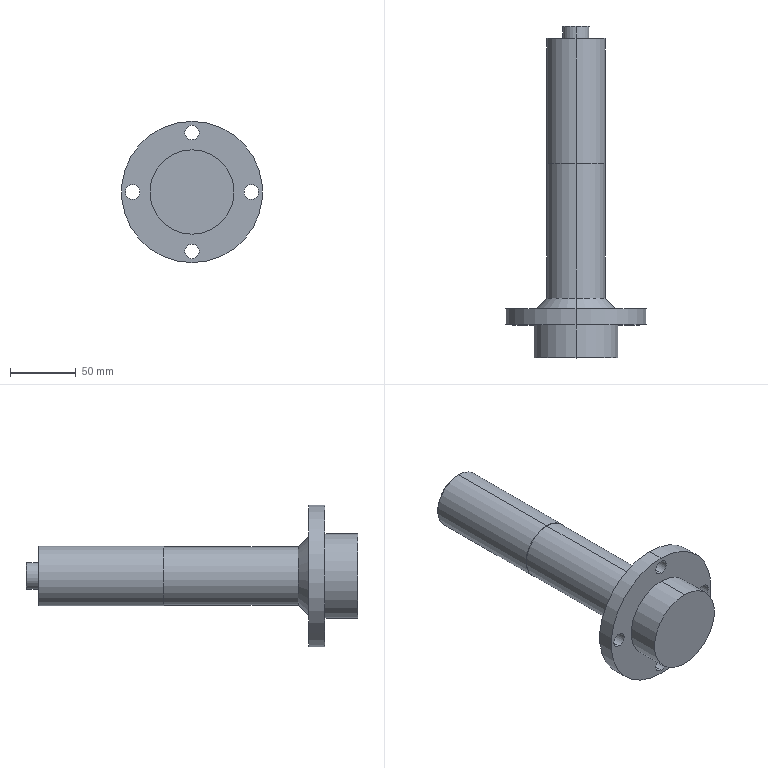Part | SolidWorks | features BaseBody 1 | 1 solid | 46 faces | box 107 x 251.6 x 107 mm | volume 513501 mm3 | cylinder 26 | cone 14 | plane 6 | commonest cylinder face diameters 5 x8 11 x8 20 x2 44.3 x2 45 x2 64 x2
STEP:
#1=CARTESIAN_POINT('',(0.,147.3,-22.15));
#2=VERTEX_POINT('',#1);
#3=CARTESIAN_POINT('',(0.,147.3,22.15));
#4=VERTEX_POINT('',#3);
#5=CARTESIAN_POINT('',(0.,147.3,0.));
#6=DIRECTION('',(0.,-1.,0.));
#7=DIRECTION('',(0.,0.,-1.));
#8=AXIS2_PLACEMENT_3D('',#5,#6,#7);
#9=CIRCLE('',#8,22.15);
#10=EDGE_CURVE('',#2,#4,#9,.T.);
#11=ORIENTED_EDGE('',*,*,#10,.T.);
#12=CARTESIAN_POINT('',(0.,45.3,22.15));
#13=VERTEX_POINT('',#12);
#14=CARTESIAN_POINT('',(0.,147.3,22.15));
#15=DIRECTION('',(0.,-1.,0.));
#16=VECTOR('',#15,1000.);
#17=LINE('',#14,#16);
#18=EDGE_CURVE('',#4,#13,#17,.T.);
#19=ORIENTED_EDGE('',*,*,#18,.T.);
#20=CARTESIAN_POINT('',(0.,45.3,-22.15));
#21=VERTEX_POINT('',#20);
#22=CARTESIAN_POINT('',(0.,45.3,0.));
#23=DIRECTION('',(0.,1.,0.));
#24=DIRECTION('',(0.,0.,-1.));
#25=AXIS2_PLACEMENT_3D('',#22,#23,#24);
#26=CIRCLE('',#25,22.15);
#27=EDGE_CURVE('',#13,#21,#26,.T.);
#28=ORIENTED_EDGE('',*,*,#27,.T.);
#29=CARTESIAN_POINT('',(0.,147.3,-22.15));
#30=DIRECTION('',(0.,-1.,0.));
#31=VECTOR('',#30,1000.);
#32=LINE('',#29,#31);
#33=EDGE_CURVE('',#2,#21,#32,.T.);
#34=ORIENTED_EDGE('',*,*,#33,.F.);
#35=EDGE_LOOP('',(#11,#19,#28,#34));
#36=FACE_OUTER_BOUND('',#35,.T.);
#37=CARTESIAN_POINT('',(0.,147.3,0.));
#38=DIRECTION('',(0.,-1.,0.));
#39=DIRECTION('',(0.,0.,-1.));
#40=AXIS2_PLACEMENT_3D('',#37,#38,#39);
#41=CYLINDRICAL_SURFACE('',#40,22.15);
#42=ADVANCED_FACE('',(#36),#41,.T.);
#43=ORIENTED_EDGE('',*,*,#27,.F.);
#44=CARTESIAN_POINT('',(0.,37.3,30.15));
#45=VERTEX_POINT('',#44);
#46=CARTESIAN_POINT('',(0.,37.3,30.15));
#47=DIRECTION('',(0.,-0.7071,0.7071));
#48=VECTOR('',#47,1000.);
#49=LINE('',#46,#48);
#50=EDGE_CURVE('',#13,#45,#49,.T.);
#51=ORIENTED_EDGE('',*,*,#50,.T.);
#52=CARTESIAN_POINT('',(0.,37.3,-30.15));
#53=VERTEX_POINT('',#52);
#54=CARTESIAN_POINT('',(0.,37.3,0.));
#55=DIRECTION('',(0.,1.,0.));
#56=DIRECTION('',(0.,0.,-1.));
#57=AXIS2_PLACEMENT_3D('',#54,#55,#56);
#58=CIRCLE('',#57,30.15);
#59=EDGE_CURVE('',#45,#53,#58,.T.);
#60=ORIENTED_EDGE('',*,*,#59,.T.);
#61=CARTESIAN_POINT('',(0.,37.3,-30.15));
#62=DIRECTION('',(0.,-0.7071,-0.7071));
#63=VECTOR('',#62,1000.);
#64=LINE('',#61,#63);
#65=EDGE_CURVE('',#21,#53,#64,.T.);
#66=ORIENTED_EDGE('',*,*,#65,.F.);
#67=EDGE_LOOP('',(#43,#51,#60,#66));
#68=FACE_OUTER_BOUND('',#67,.T.);
#69=CARTESIAN_POINT('',(0.,37.3,0.));
#70=DIRECTION('',(0.,-1.,0.));
#71=DIRECTION('',(0.,0.,-1.));
#72=AXIS2_PLACEMENT_3D('',#69,#70,#71);
#73=CONICAL_SURFACE('',#72,30.15,0.7854);
#74=ADVANCED_FACE('',(#68),#73,.T.);
#75=CARTESIAN_POINT('',(0.,241.8,-22.5));
#76=VERTEX_POINT('',#75);
#77=CARTESIAN_POINT('',(0.,241.8,22.5));
#78=VERTEX_POINT('',#77);
#79=CARTESIAN_POINT('',(0.,241.8,0.));
#80=DIRECTION('',(0.,-1.,0.));
#81=DIRECTION('',(0.,0.,-1.));
#82=AXIS2_PLACEMENT_3D('',#79,#80,#81);
#83=CIRCLE('',#82,22.5);
#84=EDGE_CURVE('',#76,#78,#83,.T.);
#85=ORIENTED_EDGE('',*,*,#84,.T.);
#86=CARTESIAN_POINT('',(0.,147.3,22.5));
#87=VERTEX_POINT('',#86);
#88=CARTESIAN_POINT('',(0.,242.3,22.5));
#89=DIRECTION('',(0.,-1.,0.));
#90=VECTOR('',#89,1000.);
#91=LINE('',#88,#90);
#92=EDGE_CURVE('',#78,#87,#91,.T.);
#93=ORIENTED_EDGE('',*,*,#92,.T.);
#94=CARTESIAN_POINT('',(0.,147.3,-22.5));
#95=VERTEX_POINT('',#94);
#96=CARTESIAN_POINT('',(0.,147.3,0.));
#97=DIRECTION('',(0.,1.,0.));
#98=DIRECTION('',(0.,0.,-1.));
#99=AXIS2_PLACEMENT_3D('',#96,#97,#98);
#100=CIRCLE('',#99,22.5);
#101=EDGE_CURVE('',#87,#95,#100,.T.);
#102=ORIENTED_EDGE('',*,*,#101,.T.);
#103=CARTESIAN_POINT('',(0.,242.3,-22.5));
#104=DIRECTION('',(0.,-1.,0.));
#105=VECTOR('',#104,1000.);
#106=LINE('',#103,#105);
#107=EDGE_CURVE('',#76,#95,#106,.T.);
#108=ORIENTED_EDGE('',*,*,#107,.F.);
#109=EDGE_LOOP('',(#85,#93,#102,#108));
#110=FACE_OUTER_BOUND('',#109,.T.);
#111=CARTESIAN_POINT('',(0.,242.3,0.));
#112=DIRECTION('',(0.,-1.,0.));
#113=DIRECTION('',(0.,0.,-1.));
#114=AXIS2_PLACEMENT_3D('',#111,#112,#113);
#115=CYLINDRICAL_SURFACE('',#114,22.5);
#116=ADVANCED_FACE('',(#110),#115,.T.);
#117=CARTESIAN_POINT('',(0.,37.3,53.5));
#118=VERTEX_POINT('',#117);
#119=CARTESIAN_POINT('',(0.,37.3,-53.5));
#120=VERTEX_POINT('',#119);
#121=CARTESIAN_POINT('',(0.,37.3,0.));
#122=DIRECTION('',(0.,1.,0.));
#123=DIRECTION('',(0.,0.,-1.));
#124=AXIS2_PLACEMENT_3D('',#121,#122,#123);
#125=CIRCLE('',#124,53.5);
#126=EDGE_CURVE('',#118,#120,#125,.T.);
#127=ORIENTED_EDGE('',*,*,#126,.F.);
#128=CARTESIAN_POINT('',(0.,25.,53.5));
#129=VERTEX_POINT('',#128);
#130=CARTESIAN_POINT('',(0.,37.3,53.5));
#131=DIRECTION('',(0.,-1.,0.));
#132=VECTOR('',#131,1000.);
#133=LINE('',#130,#132);
#134=EDGE_CURVE('',#118,#129,#133,.T.);
#135=ORIENTED_EDGE('',*,*,#134,.T.);
#136=CARTESIAN_POINT('',(0.,25.,-53.5));
#137=VERTEX_POINT('',#136);
#138=CARTESIAN_POINT('',(0.,25.,0.));
#139=DIRECTION('',(0.,1.,0.));
#140=DIRECTION('',(0.,0.,-1.));
#141=AXIS2_PLACEMENT_3D('',#138,#139,#140);
#142=CIRCLE('',#141,53.5);
#143=EDGE_CURVE('',#129,#137,#142,.T.);
#144=ORIENTED_EDGE('',*,*,#143,.T.);
#145=CARTESIAN_POINT('',(0.,37.3,-53.5));
#146=DIRECTION('',(0.,-1.,0.));
#147=VECTOR('',#146,1000.);
#148=LINE('',#145,#147);
#149=EDGE_CURVE('',#120,#137,#148,.T.);
#150=ORIENTED_EDGE('',*,*,#149,.F.);
#151=EDGE_LOOP('',(#127,#135,#144,#150));
#152=FACE_OUTER_BOUND('',#151,.T.);
#153=CARTESIAN_POINT('',(0.,37.3,0.));
#154=DIRECTION('',(0.,-1.,0.));
#155=DIRECTION('',(0.,0.,-1.));
#156=AXIS2_PLACEMENT_3D('',#153,#154,#155);
#157=CYLINDRICAL_SURFACE('',#156,53.5);
#158=ADVANCED_FACE('',(#152),#157,.T.);
#159=CARTESIAN_POINT('',(-45.,37.3,5.5));
#160=VERTEX_POINT('',#159);
#161=CARTESIAN_POINT('',(-45.,37.3,-5.5));
#162=VERTEX_POINT('',#161);
#163=CARTESIAN_POINT('',(-45.,37.3,0.));
#164=DIRECTION('',(0.,-1.,0.));
#165=DIRECTION('',(0.,0.,-1.));
#166=AXIS2_PLACEMENT_3D('',#163,#164,#165);
#167=CIRCLE('',#166,5.5);
#168=EDGE_CURVE('',#160,#162,#167,.T.);
#169=ORIENTED_EDGE('',*,*,#168,.F.);
#170=CARTESIAN_POINT('',(-45.,25.,5.5));
#171=VERTEX_POINT('',#170);
#172=CARTESIAN_POINT('',(-45.,37.3,5.5));
#173=DIRECTION('',(0.,-1.,0.));
#174=VECTOR('',#173,1000.);
#175=LINE('',#172,#174);
#176=EDGE_CURVE('',#160,#171,#175,.T.);
#177=ORIENTED_EDGE('',*,*,#176,.T.);
#178=CARTESIAN_POINT('',(-45.,25.,-5.5));
#179=VERTEX_POINT('',#178);
#180=CARTESIAN_POINT('',(-45.,25.,0.));
#181=DIRECTION('',(0.,1.,0.));
#182=DIRECTION('',(0.,0.,-1.));
#183=AXIS2_PLACEMENT_3D('',#180,#181,#182);
#184=CIRCLE('',#183,5.5);
#185=EDGE_CURVE('',#179,#171,#184,.T.);
#186=ORIENTED_EDGE('',*,*,#185,.F.);
#187=CARTESIAN_POINT('',(-45.,37.3,-5.5));
#188=DIRECTION('',(0.,-1.,0.));
#189=VECTOR('',#188,1000.);
#190=LINE('',#187,#189);
#191=EDGE_CURVE('',#162,#179,#190,.T.);
#192=ORIENTED_EDGE('',*,*,#191,.F.);
#193=EDGE_LOOP('',(#169,#177,#186,#192));
#194=FACE_OUTER_BOUND('',#193,.T.);
#195=CARTESIAN_POINT('',(-45.,37.3,0.));
#196=DIRECTION('',(0.,-1.,0.));
#197=DIRECTION('',(0.,0.,-1.));
#198=AXIS2_PLACEMENT_3D('',#195,#196,#197);
#199=CYLINDRICAL_SURFACE('',#198,5.5);
#200=ADVANCED_FACE('',(#194),#199,.F.);
#201=CARTESIAN_POINT('',(0.,37.3,-39.5));
#202=VERTEX_POINT('',#201);
#203=CARTESIAN_POINT('',(0.,37.3,-50.5));
#204=VERTEX_POINT('',#203);
#205=CARTESIAN_POINT('',(0.,37.3,-45.));
#206=DIRECTION('',(0.,-1.,0.));
#207=DIRECTION('',(0.,0.,-1.));
#208=AXIS2_PLACEMENT_3D('',#205,#206,#207);
#209=CIRCLE('',#208,5.5);
#210=EDGE_CURVE('',#202,#204,#209,.T.);
#211=ORIENTED_EDGE('',*,*,#210,.F.);
#212=CARTESIAN_POINT('',(0.,25.,-39.5));
#213=VERTEX_POINT('',#212);
#214=CARTESIAN_POINT('',(0.,37.3,-39.5));
#215=DIRECTION('',(0.,-1.,0.));
#216=VECTOR('',#215,1000.);
#217=LINE('',#214,#216);
#218=EDGE_CURVE('',#202,#213,#217,.T.);
#219=ORIENTED_EDGE('',*,*,#218,.T.);
#220=CARTESIAN_POINT('',(0.,25.,-50.5));
#221=VERTEX_POINT('',#220);
#222=CARTESIAN_POINT('',(0.,25.,-45.));
#223=DIRECTION('',(0.,1.,0.));
#224=DIRECTION('',(0.,0.,-1.));
#225=AXIS2_PLACEMENT_3D('',#222,#223,#224);
#226=CIRCLE('',#225,5.5);
#227=EDGE_CURVE('',#221,#213,#226,.T.);
#228=ORIENTED_EDGE('',*,*,#227,.F.);
#229=CARTESIAN_POINT('',(0.,37.3,-50.5));
#230=DIRECTION('',(0.,-1.,0.));
#231=VECTOR('',#230,1000.);
#232=LINE('',#229,#231);
#233=EDGE_CURVE('',#204,#221,#232,.T.);
#234=ORIENTED_EDGE('',*,*,#233,.F.);
#235=EDGE_LOOP('',(#211,#219,#228,#234));
#236=FACE_OUTER_BOUND('',#235,.T.);
#237=CARTESIAN_POINT('',(0.,37.3,-45.));
#238=DIRECTION('',(0.,-1.,0.));
#239=DIRECTION('',(0.,0.,-1.));
#240=AXIS2_PLACEMENT_3D('',#237,#238,#239);
#241=CYLINDRICAL_SURFACE('',#240,5.5);
#242=ADVANCED_FACE('',(#236),#241,.F.);
#243=CARTESIAN_POINT('',(45.,37.3,5.5));
#244=VERTEX_POINT('',#243);
#245=CARTESIAN_POINT('',(45.,37.3,-5.5));
#246=VERTEX_POINT('',#245);
#247=CARTESIAN_POINT('',(45.,37.3,0.));
#248=DIRECTION('',(0.,-1.,0.));
#249=DIRECTION('',(0.,0.,-1.));
#250=AXIS2_PLACEMENT_3D('',#247,#248,#249);
#251=CIRCLE('',#250,5.5);
#252=EDGE_CURVE('',#244,#246,#251,.T.);
#253=ORIENTED_EDGE('',*,*,#252,.F.);
#254=CARTESIAN_POINT('',(45.,25.,5.5));
#255=VERTEX_POINT('',#254);
#256=CARTESIAN_POINT('',(45.,37.3,5.5));
#257=DIRECTION('',(0.,-1.,0.));
#258=VECTOR('',#257,1000.);
#259=LINE('',#256,#258);
#260=EDGE_CURVE('',#244,#255,#259,.T.);
#261=ORIENTED_EDGE('',*,*,#260,.T.);
#262=CARTESIAN_POINT('',(45.,25.,-5.5));
#263=VERTEX_POINT('',#262);
#264=CARTESIAN_POINT('',(45.,25.,0.));
#265=DIRECTION('',(0.,1.,0.));
#266=DIRECTION('',(0.,0.,-1.));
#267=AXIS2_PLACEMENT_3D('',#264,#265,#266);
#268=CIRCLE('',#267,5.5);
#269=EDGE_CURVE('',#263,#255,#268,.T.);
#270=ORIENTED_EDGE('',*,*,#269,.F.);
#271=CARTESIAN_POINT('',(45.,37.3,-5.5));
#272=DIRECTION('',(0.,-1.,0.));
#273=VECTOR('',#272,1000.);
#274=LINE('',#271,#273);
#275=EDGE_CURVE('',#246,#263,#274,.T.);
#276=ORIENTED_EDGE('',*,*,#275,.F.);
#277=EDGE_LOOP('',(#253,#261,#270,#276));
#278=FACE_OUTER_BOUND('',#277,.T.);
#279=CARTESIAN_POINT('',(45.,37.3,0.));
#280=DIRECTION('',(0.,-1.,0.));
#281=DIRECTION('',(0.,0.,-1.));
#282=AXIS2_PLACEMENT_3D('',#279,#280,#281);
#283=CYLINDRICAL_SURFACE('',#282,5.5);
#284=ADVANCED_FACE('',(#278),#283,.F.);
#285=CARTESIAN_POINT('',(0.,37.3,50.5));
#286=VERTEX_POINT('',#285);
#287=CARTESIAN_POINT('',(0.,37.3,39.5));
#288=VERTEX_POINT('',#287);
#289=CARTESIAN_POINT('',(0.,37.3,45.));
#290=DIRECTION('',(0.,-1.,0.));
#291=DIRECTION('',(0.,0.,-1.));
#292=AXIS2_PLACEMENT_3D('',#289,#290,#291);
#293=CIRCLE('',#292,5.5);
#294=EDGE_CURVE('',#286,#288,#293,.T.);
#295=ORIENTED_EDGE('',*,*,#294,.F.);
#296=CARTESIAN_POINT('',(0.,25.,50.5));
#297=VERTEX_POINT('',#296);
#298=CARTESIAN_POINT('',(0.,37.3,50.5));
#299=DIRECTION('',(0.,-1.,0.));
#300=VECTOR('',#299,1000.);
#301=LINE('',#298,#300);
#302=EDGE_CURVE('',#286,#297,#301,.T.);
#303=ORIENTED_EDGE('',*,*,#302,.T.);
#304=CARTESIAN_POINT('',(0.,25.,39.5));
#305=VERTEX_POINT('',#304);
#306=CARTESIAN_POINT('',(0.,25.,45.));
#307=DIRECTION('',(0.,1.,0.));
#308=DIRECTION('',(0.,0.,-1.));
#309=AXIS2_PLACEMENT_3D('',#306,#307,#308);
#310=CIRCLE('',#309,5.5);
#311=EDGE_CURVE('',#305,#297,#310,.T.);
#312=ORIENTED_EDGE('',*,*,#311,.F.);
#313=CARTESIAN_POINT('',(0.,37.3,39.5));
#314=DIRECTION('',(0.,-1.,0.));
#315=VECTOR('',#314,1000.);
#316=LINE('',#313,#315);
#317=EDGE_CURVE('',#288,#305,#316,.T.);
#318=ORIENTED_EDGE('',*,*,#317,.F.);
#319=EDGE_LOOP('',(#295,#303,#312,#318));
#320=FACE_OUTER_BOUND('',#319,.T.);
#321=CARTESIAN_POINT('',(0.,37.3,45.));
#322=DIRECTION('',(0.,-1.,0.));
#323=DIRECTION('',(0.,0.,-1.));
#324=AXIS2_PLACEMENT_3D('',#321,#322,#323);
#325=CYLINDRICAL_SURFACE('',#324,5.5);
#326=ADVANCED_FACE('',(#320),#325,.F.);
#327=CARTESIAN_POINT('',(0.,242.3,-22.));
#328=VERTEX_POINT('',#327);
#329=CARTESIAN_POINT('',(0.,242.3,22.));
#330=VERTEX_POINT('',#329);
#331=CARTESIAN_POINT('',(0.,242.3,0.));
#332=DIRECTION('',(0.,-1.,0.));
#333=DIRECTION('',(0.,0.,-1.));
#334=AXIS2_PLACEMENT_3D('',#331,#332,#333);
#335=CIRCLE('',#334,22.);
#336=EDGE_CURVE('',#328,#330,#335,.T.);
#337=ORIENTED_EDGE('',*,*,#336,.T.);
#338=CARTESIAN_POINT('',(0.,241.8,22.5));
#339=DIRECTION('',(0.,-0.7071,0.7071));
#340=VECTOR('',#339,1000.);
#341=LINE('',#338,#340);
#342=EDGE_CURVE('',#330,#78,#341,.T.);
#343=ORIENTED_EDGE('',*,*,#342,.T.);
#344=ORIENTED_EDGE('',*,*,#84,.F.);
#345=CARTESIAN_POINT('',(0.,241.8,-22.5));
#346=DIRECTION('',(0.,-0.7071,-0.7071));
#347=VECTOR('',#346,1000.);
#348=LINE('',#345,#347);
#349=EDGE_CURVE('',#328,#76,#348,.T.);
#350=ORIENTED_EDGE('',*,*,#349,.F.);
#351=EDGE_LOOP('',(#337,#343,#344,#350));
#352=FACE_OUTER_BOUND('',#351,.T.);
#353=CARTESIAN_POINT('',(0.,241.8,0.));
#354=DIRECTION('',(0.,-1.,0.));
#355=DIRECTION('',(0.,0.,-1.));
#356=AXIS2_PLACEMENT_3D('',#353,#354,#355);
#357=CONICAL_SURFACE('',#356,22.5,0.7854);
#358=ADVANCED_FACE('',(#352),#357,.T.);
#359=CARTESIAN_POINT('',(0.,25.,-32.));
#360=VERTEX_POINT('',#359);
#361=CARTESIAN_POINT('',(0.,25.,32.));
#362=VERTEX_POINT('',#361);
#363=CARTESIAN_POINT('',(0.,25.,0.));
#364=DIRECTION('',(0.,-1.,0.));
#365=DIRECTION('',(0.,0.,-1.));
#366=AXIS2_PLACEMENT_3D('',#363,#364,#365);
#367=CIRCLE('',#366,32.);
#368=EDGE_CURVE('',#360,#362,#367,.T.);
#369=ORIENTED_EDGE('',*,*,#368,.T.);
#370=CARTESIAN_POINT('',(0.,0.,32.));
#371=VERTEX_POINT('',#370);
#372=CARTESIAN_POINT('',(0.,25.,32.));
#373=DIRECTION('',(0.,-1.,0.));
#374=VECTOR('',#373,1000.);
#375=LINE('',#372,#374);
#376=EDGE_CURVE('',#362,#371,#375,.T.);
#377=ORIENTED_EDGE('',*,*,#376,.T.);
#378=CARTESIAN_POINT('',(0.,0.,-32.));
#379=VERTEX_POINT('',#378);
#380=CARTESIAN_POINT('',(0.,0.,0.));
#381=DIRECTION('',(0.,1.,0.));
#382=DIRECTION('',(0.,0.,-1.));
#383=AXIS2_PLACEMENT_3D('',#380,#381,#382);
#384=CIRCLE('',#383,32.);
#385=EDGE_CURVE('',#371,#379,#384,.T.);
#386=ORIENTED_EDGE('',*,*,#385,.T.);
#387=CARTESIAN_POINT('',(0.,25.,-32.));
#388=DIRECTION('',(0.,-1.,0.));
#389=VECTOR('',#388,1000.);
#390=LINE('',#387,#389);
#391=EDGE_CURVE('',#360,#379,#390,.T.);
#392=ORIENTED_EDGE('',*,*,#391,.F.);
#393=EDGE_LOOP('',(#369,#377,#386,#392));
#394=FACE_OUTER_BOUND('',#393,.T.);
#395=CARTESIAN_POINT('',(0.,25.,0.));
#396=DIRECTION('',(0.,-1.,0.));
#397=DIRECTION('',(0.,0.,-1.));
#398=AXIS2_PLACEMENT_3D('',#395,#396,#397);
#399=CYLINDRICAL_SURFACE('',#398,32.);
#400=ADVANCED_FACE('',(#394),#399,.T.);
#401=CARTESIAN_POINT('',(0.,251.1,-10.));
#402=VERTEX_POINT('',#401);
#403=CARTESIAN_POINT('',(0.,251.1,10.));
#404=VERTEX_POINT('',#403);
#405=CARTESIAN_POINT('',(0.,251.1,0.));
#406=DIRECTION('',(0.,-1.,0.));
#407=DIRECTION('',(0.,0.,-1.));
#408=AXIS2_PLACEMENT_3D('',#405,#406,#407);
#409=CIRCLE('',#408,10.);
#410=EDGE_CURVE('',#402,#404,#409,.T.);
#411=ORIENTED_EDGE('',*,*,#410,.T.);
#412=CARTESIAN_POINT('',(0.,242.3,10.));
#413=VERTEX_POINT('',#412);
#414=CARTESIAN_POINT('',(0.,251.6,10.));
#415=DIRECTION('',(0.,-1.,0.));
#416=VECTOR('',#415,1000.);
#417=LINE('',#414,#416);
#418=EDGE_CURVE('',#404,#413,#417,.T.);
#419=ORIENTED_EDGE('',*,*,#418,.T.);
#420=CARTESIAN_POINT('',(0.,242.3,-10.));
#421=VERTEX_POINT('',#420);
#422=CARTESIAN_POINT('',(0.,242.3,0.));
#423=DIRECTION('',(0.,-1.,0.));
#424=DIRECTION('',(0.,0.,-1.));
#425=AXIS2_PLACEMENT_3D('',#422,#423,#424);
#426=CIRCLE('',#425,10.);
#427=EDGE_CURVE('',#421,#413,#426,.T.);
#428=ORIENTED_EDGE('',*,*,#427,.F.);
#429=CARTESIAN_POINT('',(0.,251.6,-10.));
#430=DIRECTION('',(0.,-1.,0.));
#431=VECTOR('',#430,1000.);
#432=LINE('',#429,#431);
#433=EDGE_CURVE('',#402,#421,#432,.T.);
#434=ORIENTED_EDGE('',*,*,#433,.F.);
#435=EDGE_LOOP('',(#411,#419,#428,#434));
#436=FACE_OUTER_BOUND('',#435,.T.);
#437=CARTESIAN_POINT('',(0.,251.6,0.));
#438=DIRECTION('',(0.,-1.,0.));
#439=DIRECTION('',(0.,0.,-1.));
#440=AXIS2_PLACEMENT_3D('',#437,#438,#439);
#441=CYLINDRICAL_SURFACE('',#440,10.);
#442=ADVANCED_FACE('',(#436),#441,.T.);
#443=CARTESIAN_POINT('',(0.,225.3,-20.));
#444=VERTEX_POINT('',#443);
#445=CARTESIAN_POINT('',(-2.5,225.3,-17.5));
#446=VERTEX_POINT('',#445);
#447=CARTESIAN_POINT('',(0.,225.3,-17.5));
#448=DIRECTION('',(0.,1.,0.));
#449=DIRECTION('',(0.,0.,1.));
#450=AXIS2_PLACEMENT_3D('',#447,#448,#449);
#451=CIRCLE('',#450,2.5);
#452=EDGE_CURVE('',#444,#446,#451,.T.);
#453=ORIENTED_EDGE('',*,*,#452,.F.);
#454=CARTESIAN_POINT('',(0.,242.3,-20.));
#455=VERTEX_POINT('',#454);
#456=CARTESIAN_POINT('',(0.,242.3,-20.));
#457=DIRECTION('',(0.,1.,0.));
#458=VECTOR('',#457,1000.);
#459=LINE('',#456,#458);
#460=EDGE_CURVE('',#444,#455,#459,.T.);
#461=ORIENTED_EDGE('',*,*,#460,.T.);
#462=CARTESIAN_POINT('',(0.,242.3,-15.));
#463=VERTEX_POINT('',#462);
#464=CARTESIAN_POINT('',(0.,242.3,-17.5));
#465=DIRECTION('',(0.,-1.,0.));
#466=DIRECTION('',(0.,0.,1.));
#467=AXIS2_PLACEMENT_3D('',#464,#465,#466);
#468=CIRCLE('',#467,2.5);
#469=EDGE_CURVE('',#463,#455,#468,.T.);
#470=ORIENTED_EDGE('',*,*,#469,.F.);
#471=CARTESIAN_POINT('',(0.,225.3,-15.));
#472=VERTEX_POINT('',#471);
#473=CARTESIAN_POINT('',(0.,242.3,-15.));
#474=DIRECTION('',(0.,1.,0.));
#475=VECTOR('',#474,1000.);
#476=LINE('',#473,#475);
#477=EDGE_CURVE('',#472,#463,#476,.T.);
#478=ORIENTED_EDGE('',*,*,#477,.F.);
#479=CARTESIAN_POINT('',(0.,225.3,-17.5));
#480=DIRECTION('',(0.,1.,0.));
#481=DIRECTION('',(0.,0.,1.));
#482=AXIS2_PLACEMENT_3D('',#479,#480,#481);
#483=CIRCLE('',#482,2.5);
#484=EDGE_CURVE('',#446,#472,#483,.T.);
#485=ORIENTED_EDGE('',*,*,#484,.F.);
#486=EDGE_LOOP('',(#453,#461,#470,#478,#485));
#487=FACE_OUTER_BOUND('',#486,.T.);
#488=CARTESIAN_POINT('',(0.,242.3,-17.5));
#489=DIRECTION('',(0.,1.,0.));
#490=DIRECTION('',(0.,0.,1.));
#491=AXIS2_PLACEMENT_3D('',#488,#489,#490);
#492=CYLINDRICAL_SURFACE('',#491,2.5);
#493=ADVANCED_FACE('',(#487),#492,.F.);
#494=CARTESIAN_POINT('',(17.5,225.3,-2.5));
#495=VERTEX_POINT('',#494);
#496=CARTESIAN_POINT('',(17.5,225.3,2.5));
#497=VERTEX_POINT('',#496);
#498=CARTESIAN_POINT('',(17.5,225.3,0.));
#499=DIRECTION('',(0.,1.,0.));
#500=DIRECTION('',(0.,0.,1.));
#501=AXIS2_PLACEMENT_3D('',#498,#499,#500);
#502=CIRCLE('',#501,2.5);
#503=EDGE_CURVE('',#495,#497,#502,.T.);
#504=ORIENTED_EDGE('',*,*,#503,.F.);
#505=CARTESIAN_POINT('',(17.5,242.3,-2.5));
#506=VERTEX_POINT('',#505);
#507=CARTESIAN_POINT('',(17.5,242.3,-2.5));
#508=DIRECTION('',(0.,1.,0.));
#509=VECTOR('',#508,1000.);
#510=LINE('',#507,#509);
#511=EDGE_CURVE('',#495,#506,#510,.T.);
#512=ORIENTED_EDGE('',*,*,#511,.T.);
#513=CARTESIAN_POINT('',(17.5,242.3,2.5));
#514=VERTEX_POINT('',#513);
#515=CARTESIAN_POINT('',(17.5,242.3,0.));
#516=DIRECTION('',(0.,-1.,0.));
#517=DIRECTION('',(0.,0.,1.));
#518=AXIS2_PLACEMENT_3D('',#515,#516,#517);
#519=CIRCLE('',#518,2.5);
#520=EDGE_CURVE('',#514,#506,#519,.T.);
#521=ORIENTED_EDGE('',*,*,#520,.F.);
#522=CARTESIAN_POINT('',(17.5,242.3,2.5));
#523=DIRECTION('',(0.,1.,0.));
#524=VECTOR('',#523,1000.);
#525=LINE('',#522,#524);
#526=EDGE_CURVE('',#497,#514,#525,.T.);
#527=ORIENTED_EDGE('',*,*,#526,.F.);
#528=EDGE_LOOP('',(#504,#512,#521,#527));
#529=FACE_OUTER_BOUND('',#528,.T.);
#530=CARTESIAN_POINT('',(17.5,242.3,0.));
#531=DIRECTION('',(0.,1.,0.));
#532=DIRECTION('',(0.,0.,1.));
#533=AXIS2_PLACEMENT_3D('',#530,#531,#532);
#534=CYLINDRICAL_SURFACE('',#533,2.5);
#535=ADVANCED_FACE('',(#529),#534,.F.);
#536=CARTESIAN_POINT('',(0.,225.3,15.));
#537=VERTEX_POINT('',#536);
#538=CARTESIAN_POINT('',(-2.5,225.3,17.5));
#539=VERTEX_POINT('',#538);
#540=CARTESIAN_POINT('',(0.,225.3,17.5));
#541=DIRECTION('',(0.,1.,0.));
#542=DIRECTION('',(0.,0.,1.));
#543=AXIS2_PLACEMENT_3D('',#540,#541,#542);
#544=CIRCLE('',#543,2.5);
#545=EDGE_CURVE('',#537,#539,#544,.T.);
#546=ORIENTED_EDGE('',*,*,#545,.F.);
#547=CARTESIAN_POINT('',(0.,242.3,15.));
#548=VERTEX_POINT('',#547);
#549=CARTESIAN_POINT('',(0.,242.3,15.));
#550=DIRECTION('',(0.,1.,0.));
#551=VECTOR('',#550,1000.);
#552=LINE('',#549,#551);
#553=EDGE_CURVE('',#537,#548,#552,.T.);
#554=ORIENTED_EDGE('',*,*,#553,.T.);
#555=CARTESIAN_POINT('',(0.,242.3,20.));
#556=VERTEX_POINT('',#555);
#557=CARTESIAN_POINT('',(0.,242.3,17.5));
#558=DIRECTION('',(0.,-1.,0.));
#559=DIRECTION('',(0.,0.,1.));
#560=AXIS2_PLACEMENT_3D('',#557,#558,#559);
#561=CIRCLE('',#560,2.5);
#562=EDGE_CURVE('',#556,#548,#561,.T.);
#563=ORIENTED_EDGE('',*,*,#562,.F.);
#564=CARTESIAN_POINT('',(0.,225.3,20.));
#565=VERTEX_POINT('',#564);
#566=CARTESIAN_POINT('',(0.,242.3,20.));
#567=DIRECTION('',(0.,1.,0.));
#568=VECTOR('',#567,1000.);
#569=LINE('',#566,#568);
#570=EDGE_CURVE('',#565,#556,#569,.T.);
#571=ORIENTED_EDGE('',*,*,#570,.F.);
#572=CARTESIAN_POINT('',(0.,225.3,17.5));
#573=DIRECTION('',(0.,1.,0.));
#574=DIRECTION('',(0.,0.,1.));
#575=AXIS2_PLACEMENT_3D('',#572,#573,#574);
#576=CIRCLE('',#575,2.5);
#577=EDGE_CURVE('',#539,#565,#576,.T.);
#578=ORIENTED_EDGE('',*,*,#577,.F.);
#579=EDGE_LOOP('',(#546,#554,#563,#571,#578));
#580=FACE_OUTER_BOUND('',#579,.T.);
#581=CARTESIAN_POINT('',(0.,242.3,17.5));
#582=DIRECTION('',(0.,1.,0.));
#583=DIRECTION('',(0.,0.,1.));
#584=AXIS2_PLACEMENT_3D('',#581,#582,#583);
#585=CYLINDRICAL_SURFACE('',#584,2.5);
#586=ADVANCED_FACE('',(#580),#585,.F.);
#587=CARTESIAN_POINT('',(-17.5,225.3,-2.5));
#588=VERTEX_POINT('',#587);
#589=CARTESIAN_POINT('',(-20.,225.3,0.));
#590=VERTEX_POINT('',#589);
#591=CARTESIAN_POINT('',(-17.5,225.3,0.));
#592=DIRECTION('',(0.,1.,0.));
#593=DIRECTION('',(0.,0.,1.));
#594=AXIS2_PLACEMENT_3D('',#591,#592,#593);
#595=CIRCLE('',#594,2.5);
#596=EDGE_CURVE('',#588,#590,#595,.T.);
#597=ORIENTED_EDGE('',*,*,#596,.F.);
#598=CARTESIAN_POINT('',(-17.5,242.3,-2.5));
#599=VERTEX_POINT('',#598);
#600=CARTESIAN_POINT('',(-17.5,242.3,-2.5));
#601=DIRECTION('',(0.,1.,0.));
#602=VECTOR('',#601,1000.);
#603=LINE('',#600,#602);
#604=EDGE_CURVE('',#588,#599,#603,.T.);
#605=ORIENTED_EDGE('',*,*,#604,.T.);
#606=CARTESIAN_POINT('',(-17.5,242.3,2.5));
#607=VERTEX_POINT('',#606);
#608=CARTESIAN_POINT('',(-17.5,242.3,0.));
#609=DIRECTION('',(0.,-1.,0.));
#610=DIRECTION('',(0.,0.,1.));
#611=AXIS2_PLACEMENT_3D('',#608,#609,#610);
#612=CIRCLE('',#611,2.5);
#613=EDGE_CURVE('',#607,#599,#612,.T.);
#614=ORIENTED_EDGE('',*,*,#613,.F.);
#615=CARTESIAN_POINT('',(-17.5,225.3,2.5));
#616=VERTEX_POINT('',#615);
#617=CARTESIAN_POINT('',(-17.5,242.3,2.5));
#618=DIRECTION('',(0.,1.,0.));
#619=VECTOR('',#618,1000.);
#620=LINE('',#617,#619);
#621=EDGE_CURVE('',#616,#607,#620,.T.);
#622=ORIENTED_EDGE('',*,*,#621,.F.);
#623=CARTESIAN_POINT('',(-17.5,225.3,0.));
#624=DIRECTION('',(0.,1.,0.));
#625=DIRECTION('',(0.,0.,1.));
#626=AXIS2_PLACEMENT_3D('',#623,#624,#625);
#627=CIRCLE('',#626,2.5);
#628=EDGE_CURVE('',#590,#616,#627,.T.);
#629=ORIENTED_EDGE('',*,*,#628,.F.);
#630=EDGE_LOOP('',(#597,#605,#614,#622,#629));
#631=FACE_OUTER_BOUND('',#630,.T.);
#632=CARTESIAN_POINT('',(-17.5,242.3,0.));
#633=DIRECTION('',(0.,1.,0.));
#634=DIRECTION('',(0.,0.,1.));
#635=AXIS2_PLACEMENT_3D('',#632,#633,#634);
#636=CYLINDRICAL_SURFACE('',#635,2.5);
#637=ADVANCED_FACE('',(#631),#636,.F.);
#638=CARTESIAN_POINT('',(0.,251.6,-9.5));
#639=VERTEX_POINT('',#638);
#640=CARTESIAN_POINT('',(0.,251.6,9.5));
#641=VERTEX_POINT('',#640);
#642=CARTESIAN_POINT('',(0.,251.6,0.));
#643=DIRECTION('',(0.,-1.,0.));
#644=DIRECTION('',(0.,0.,-1.));
#645=AXIS2_PLACEMENT_3D('',#642,#643,#644);
#646=CIRCLE('',#645,9.5);
#647=EDGE_CURVE('',#639,#641,#646,.T.);
#648=ORIENTED_EDGE('',*,*,#647,.T.);
#649=CARTESIAN_POINT('',(0.,251.1,10.));
#650=DIRECTION('',(0.,-0.7071,0.7071));
#651=VECTOR('',#650,1000.);
#652=LINE('',#649,#651);
#653=EDGE_CURVE('',#641,#404,#652,.T.);
#654=ORIENTED_EDGE('',*,*,#653,.T.);
#655=ORIENTED_EDGE('',*,*,#410,.F.);
#656=CARTESIAN_POINT('',(0.,251.1,-10.));
#657=DIRECTION('',(0.,-0.7071,-0.7071));
#658=VECTOR('',#657,1000.);
#659=LINE('',#656,#658);
#660=EDGE_CURVE('',#639,#402,#659,.T.);
#661=ORIENTED_EDGE('',*,*,#660,.F.);
#662=EDGE_LOOP('',(#648,#654,#655,#661));
#663=FACE_OUTER_BOUND('',#662,.T.);
#664=CARTESIAN_POINT('',(0.,251.1,0.));
#665=DIRECTION('',(0.,-1.,0.));
#666=DIRECTION('',(0.,0.,-1.));
#667=AXIS2_PLACEMENT_3D('',#664,#665,#666);
#668=CONICAL_SURFACE('',#667,10.,0.7854);
#669=ADVANCED_FACE('',(#663),#668,.T.);
#670=CARTESIAN_POINT('',(0.,223.798,-17.5));
#671=VERTEX_POINT('',#670);
#672=CARTESIAN_POINT('',(-2.5,225.3,-17.5));
#673=DIRECTION('',(-0.8572,0.515,0.));
#674=VECTOR('',#673,1000.);
#675=LINE('',#672,#674);
#676=EDGE_CURVE('',#671,#446,#675,.T.);
#677=ORIENTED_EDGE('',*,*,#676,.F.);
#678=CARTESIAN_POINT('',(2.5,225.3,-17.5));
#679=VERTEX_POINT('',#678);
#680=CARTESIAN_POINT('',(2.5,225.3,-17.5));
#681=DIRECTION('',(0.8572,0.515,0.));
#682=VECTOR('',#681,1000.);
#683=LINE('',#680,#682);
#684=EDGE_CURVE('',#671,#679,#683,.T.);
#685=ORIENTED_EDGE('',*,*,#684,.T.);
#686=CARTESIAN_POINT('',(0.,225.3,-17.5));
#687=DIRECTION('',(0.,1.,0.));
#688=DIRECTION('',(0.,0.,1.));
#689=AXIS2_PLACEMENT_3D('',#686,#687,#688);
#690=CIRCLE('',#689,2.5);
#691=EDGE_CURVE('',#679,#444,#690,.T.);
#692=ORIENTED_EDGE('',*,*,#691,.T.);
#693=ORIENTED_EDGE('',*,*,#452,.T.);
#694=EDGE_LOOP('',(#677,#685,#692,#693));
#695=FACE_OUTER_BOUND('',#694,.T.);
#696=CARTESIAN_POINT('',(0.,225.3,-17.5));
#697=DIRECTION('',(0.,1.,0.));
#698=DIRECTION('',(-1.,0.,0.));
#699=AXIS2_PLACEMENT_3D('',#696,#697,#698);
#700=CONICAL_SURFACE('',#699,2.5,1.03);
#701=ADVANCED_FACE('',(#695),#700,.F.);
#702=CARTESIAN_POINT('',(17.5,223.798,0.));
#703=VERTEX_POINT('',#702);
#704=CARTESIAN_POINT('',(17.5,225.3,2.5));
#705=DIRECTION('',(0.,0.515,0.8572));
#706=VECTOR('',#705,1000.);
#707=LINE('',#704,#706);
#708=EDGE_CURVE('',#703,#497,#707,.T.);
#709=ORIENTED_EDGE('',*,*,#708,.F.);
#710=CARTESIAN_POINT('',(17.5,225.3,-2.5));
#711=DIRECTION('',(0.,0.515,-0.8572));
#712=VECTOR('',#711,1000.);
#713=LINE('',#710,#712);
#714=EDGE_CURVE('',#703,#495,#713,.T.);
#715=ORIENTED_EDGE('',*,*,#714,.T.);
#716=ORIENTED_EDGE('',*,*,#503,.T.);
#717=EDGE_LOOP('',(#709,#715,#716));
#718=FACE_OUTER_BOUND('',#717,.T.);
#719=CARTESIAN_POINT('',(17.5,225.3,0.));
#720=DIRECTION('',(0.,1.,0.));
#721=DIRECTION('',(0.,0.,1.));
#722=AXIS2_PLACEMENT_3D('',#719,#720,#721);
#723=CONICAL_SURFACE('',#722,2.5,1.03);
#724=ADVANCED_FACE('',(#718),#723,.F.);
#725=CARTESIAN_POINT('',(0.,223.798,17.5));
#726=VERTEX_POINT('',#725);
#727=CARTESIAN_POINT('',(-2.5,225.3,17.5));
#728=DIRECTION('',(-0.8572,0.515,0.));
#729=VECTOR('',#728,1000.);
#730=LINE('',#727,#729);
#731=EDGE_CURVE('',#726,#539,#730,.T.);
#732=ORIENTED_EDGE('',*,*,#731,.F.);
#733=CARTESIAN_POINT('',(2.5,225.3,17.5));
#734=VERTEX_POINT('',#733);
#735=CARTESIAN_POINT('',(2.5,225.3,17.5));
#736=DIRECTION('',(0.8572,0.515,0.));
#737=VECTOR('',#736,1000.);
#738=LINE('',#735,#737);
#739=EDGE_CURVE('',#726,#734,#738,.T.);
#740=ORIENTED_EDGE('',*,*,#739,.T.);
#741=CARTESIAN_POINT('',(0.,225.3,17.5));
#742=DIRECTION('',(0.,1.,0.));
#743=DIRECTION('',(0.,0.,1.));
#744=AXIS2_PLACEMENT_3D('',#741,#742,#743);
#745=CIRCLE('',#744,2.5);
#746=EDGE_CURVE('',#734,#537,#745,.T.);
#747=ORIENTED_EDGE('',*,*,#746,.T.);
#748=ORIENTED_EDGE('',*,*,#545,.T.);
#749=EDGE_LOOP('',(#732,#740,#747,#748));
#750=FACE_OUTER_BOUND('',#749,.T.);
#751=CARTESIAN_POINT('',(0.,225.3,17.5));
#752=DIRECTION('',(0.,1.,0.));
#753=DIRECTION('',(-1.,0.,0.));
#754=AXIS2_PLACEMENT_3D('',#751,#752,#753);
#755=CONICAL_SURFACE('',#754,2.5,1.03);
#756=ADVANCED_FACE('',(#750),#755,.F.);
#757=CARTESIAN_POINT('',(-17.5,223.798,0.));
#758=VERTEX_POINT('',#757);
#759=CARTESIAN_POINT('',(-20.,225.3,0.));
#760=DIRECTION('',(-0.8572,0.515,0.));
#761=VECTOR('',#760,1000.);
#762=LINE('',#759,#761);
#763=EDGE_CURVE('',#758,#590,#762,.T.);
#764=ORIENTED_EDGE('',*,*,#763,.F.);
#765=CARTESIAN_POINT('',(-15.,225.3,0.));
#766=VERTEX_POINT('',#765);
#767=CARTESIAN_POINT('',(-15.,225.3,0.));
#768=DIRECTION('',(0.8572,0.515,0.));
#769=VECTOR('',#768,1000.);
#770=LINE('',#767,#769);
#771=EDGE_CURVE('',#758,#766,#770,.T.);
#772=ORIENTED_EDGE('',*,*,#771,.T.);
#773=CARTESIAN_POINT('',(-17.5,225.3,0.));
#774=DIRECTION('',(0.,1.,0.));
#775=DIRECTION('',(0.,0.,1.));
#776=AXIS2_PLACEMENT_3D('',#773,#774,#775);
#777=CIRCLE('',#776,2.5);
#778=EDGE_CURVE('',#766,#588,#777,.T.);
#779=ORIENTED_EDGE('',*,*,#778,.T.);
#780=ORIENTED_EDGE('',*,*,#596,.T.);
#781=EDGE_LOOP('',(#764,#772,#779,#780));
#782=FACE_OUTER_BOUND('',#781,.T.);
#783=CARTESIAN_POINT('',(-17.5,225.3,0.));
#784=DIRECTION('',(0.,1.,0.));
#785=DIRECTION('',(-1.,0.,0.));
#786=AXIS2_PLACEMENT_3D('',#783,#784,#785);
#787=CONICAL_SURFACE('',#786,2.5,1.03);
#788=ADVANCED_FACE('',(#782),#787,.F.);
#789=ORIENTED_EDGE('',*,*,#18,.F.);
#790=CARTESIAN_POINT('',(0.,147.3,0.));
#791=DIRECTION('',(0.,-1.,0.));
#792=DIRECTION('',(0.,0.,-1.));
#793=AXIS2_PLACEMENT_3D('',#790,#791,#792);
#794=CIRCLE('',#793,22.15);
#795=EDGE_CURVE('',#4,#2,#794,.T.);
#796=ORIENTED_EDGE('',*,*,#795,.T.);
#797=ORIENTED_EDGE('',*,*,#33,.T.);
#798=CARTESIAN_POINT('',(0.,45.3,0.));
#799=DIRECTION('',(0.,1.,0.));
#800=DIRECTION('',(0.,0.,-1.));
#801=AXIS2_PLACEMENT_3D('',#798,#799,#800);
#802=CIRCLE('',#801,22.15);
#803=EDGE_CURVE('',#21,#13,#802,.T.);
#804=ORIENTED_EDGE('',*,*,#803,.T.);
#805=EDGE_LOOP('',(#789,#796,#797,#804));
#806=FACE_OUTER_BOUND('',#805,.T.);
#807=CARTESIAN_POINT('',(0.,147.3,0.));
#808=DIRECTION('',(0.,-1.,0.));
#809=DIRECTION('',(0.,0.,-1.));
#810=AXIS2_PLACEMENT_3D('',#807,#808,#809);
#811=CYLINDRICAL_SURFACE('',#810,22.15);
#812=ADVANCED_FACE('',(#806),#811,.T.);
#813=ORIENTED_EDGE('',*,*,#50,.F.);
#814=ORIENTED_EDGE('',*,*,#803,.F.);
#815=ORIENTED_EDGE('',*,*,#65,.T.);
#816=CARTESIAN_POINT('',(0.,37.3,0.));
#817=DIRECTION('',(0.,1.,0.));
#818=DIRECTION('',(0.,0.,-1.));
#819=AXIS2_PLACEMENT_3D('',#816,#817,#818);
#820=CIRCLE('',#819,30.15);
#821=EDGE_CURVE('',#53,#45,#820,.T.);
#822=ORIENTED_EDGE('',*,*,#821,.T.);
#823=EDGE_LOOP('',(#813,#814,#815,#822));
#824=FACE_OUTER_BOUND('',#823,.T.);
#825=CARTESIAN_POINT('',(0.,37.3,0.));
#826=DIRECTION('',(0.,-1.,0.));
#827=DIRECTION('',(0.,0.,-1.));
#828=AXIS2_PLACEMENT_3D('',#825,#826,#827);
#829=CONICAL_SURFACE('',#828,30.15,0.7854);
#830=ADVANCED_FACE('',(#824),#829,.T.);
#831=CARTESIAN_POINT('',(0.,147.3,0.));
#832=DIRECTION('',(0.,1.,0.));
#833=DIRECTION('',(0.,0.,-1.));
#834=AXIS2_PLACEMENT_3D('',#831,#832,#833);
#835=CIRCLE('',#834,22.5);
#836=EDGE_CURVE('',#95,#87,#835,.T.);
#837=ORIENTED_EDGE('',*,*,#836,.F.);
#838=ORIENTED_EDGE('',*,*,#101,.F.);
#839=EDGE_LOOP('',(#837,#838));
#840=FACE_OUTER_BOUND('',#839,.T.);
#841=ORIENTED_EDGE('',*,*,#10,.F.);
#842=ORIENTED_EDGE('',*,*,#795,.F.);
#843=EDGE_LOOP('',(#841,#842));
#844=FACE_BOUND('',#843,.T.);
#845=CARTESIAN_POINT('',(0.,147.3,0.));
#846=DIRECTION('',(0.,1.,0.));
#847=DIRECTION('',(0.,0.,1.));
#848=AXIS2_PLACEMENT_3D('',#845,#846,#847);
#849=PLANE('',#848);
#850=ADVANCED_FACE('',(#840,#844),#849,.F.);
#851=CARTESIAN_POINT('',(0.,37.3,0.));
#852=DIRECTION('',(0.,1.,0.));
#853=DIRECTION('',(0.,0.,-1.));
#854=AXIS2_PLACEMENT_3D('',#851,#852,#853);
#855=CIRCLE('',#854,53.5);
#856=EDGE_CURVE('',#120,#118,#855,.T.);
#857=ORIENTED_EDGE('',*,*,#856,.T.);
#858=ORIENTED_EDGE('',*,*,#126,.T.);
#859=EDGE_LOOP('',(#857,#858));
#860=FACE_OUTER_BOUND('',#859,.T.);
#861=CARTESIAN_POINT('',(-45.,37.3,0.));
#862=DIRECTION('',(0.,-1.,0.));
#863=DIRECTION('',(0.,0.,-1.));
#864=AXIS2_PLACEMENT_3D('',#861,#862,#863);
#865=CIRCLE('',#864,5.5);
#866=EDGE_CURVE('',#162,#160,#865,.T.);
#867=ORIENTED_EDGE('',*,*,#866,.T.);
#868=ORIENTED_EDGE('',*,*,#168,.T.);
#869=EDGE_LOOP('',(#867,#868));
#870=FACE_BOUND('',#869,.T.);
#871=CARTESIAN_POINT('',(0.,37.3,-45.));
#872=DIRECTION('',(0.,-1.,0.));
#873=DIRECTION('',(0.,0.,-1.));
#874=AXIS2_PLACEMENT_3D('',#871,#872,#873);
#875=CIRCLE('',#874,5.5);
#876=EDGE_CURVE('',#204,#202,#875,.T.);
#877=ORIENTED_EDGE('',*,*,#876,.T.);
#878=ORIENTED_EDGE('',*,*,#210,.T.);
#879=EDGE_LOOP('',(#877,#878));
#880=FACE_BOUND('',#879,.T.);
#881=CARTESIAN_POINT('',(45.,37.3,0.));
#882=DIRECTION('',(0.,-1.,0.));
#883=DIRECTION('',(0.,0.,-1.));
#884=AXIS2_PLACEMENT_3D('',#881,#882,#883);
#885=CIRCLE('',#884,5.5);
#886=EDGE_CURVE('',#246,#244,#885,.T.);
#887=ORIENTED_EDGE('',*,*,#886,.T.);
#888=ORIENTED_EDGE('',*,*,#252,.T.);
#889=EDGE_LOOP('',(#887,#888));
#890=FACE_BOUND('',#889,.T.);
#891=CARTESIAN_POINT('',(0.,37.3,45.));
#892=DIRECTION('',(0.,-1.,0.));
#893=DIRECTION('',(0.,0.,-1.));
#894=AXIS2_PLACEMENT_3D('',#891,#892,#893);
#895=CIRCLE('',#894,5.5);
#896=EDGE_CURVE('',#288,#286,#895,.T.);
#897=ORIENTED_EDGE('',*,*,#896,.T.);
#898=ORIENTED_EDGE('',*,*,#294,.T.);
#899=EDGE_LOOP('',(#897,#898));
#900=FACE_BOUND('',#899,.T.);
#901=ORIENTED_EDGE('',*,*,#821,.F.);
#902=ORIENTED_EDGE('',*,*,#59,.F.);
#903=EDGE_LOOP('',(#901,#902));
#904=FACE_BOUND('',#903,.T.);
#905=CARTESIAN_POINT('',(0.,37.3,0.));
#906=DIRECTION('',(0.,1.,0.));
#907=DIRECTION('',(0.,0.,1.));
#908=AXIS2_PLACEMENT_3D('',#905,#906,#907);
#909=PLANE('',#908);
#910=ADVANCED_FACE('',(#860,#870,#880,#890,#900,#904),#909,.T.);
#911=ORIENTED_EDGE('',*,*,#92,.F.);
#912=CARTESIAN_POINT('',(0.,241.8,0.));
#913=DIRECTION('',(0.,-1.,0.));
#914=DIRECTION('',(0.,0.,-1.));
#915=AXIS2_PLACEMENT_3D('',#912,#913,#914);
#916=CIRCLE('',#915,22.5);
#917=EDGE_CURVE('',#78,#76,#916,.T.);
#918=ORIENTED_EDGE('',*,*,#917,.T.);
#919=ORIENTED_EDGE('',*,*,#107,.T.);
#920=ORIENTED_EDGE('',*,*,#836,.T.);
#921=EDGE_LOOP('',(#911,#918,#919,#920));
#922=FACE_OUTER_BOUND('',#921,.T.);
#923=CARTESIAN_POINT('',(0.,242.3,0.));
#924=DIRECTION('',(0.,-1.,0.));
#925=DIRECTION('',(0.,0.,-1.));
#926=AXIS2_PLACEMENT_3D('',#923,#924,#925);
#927=CYLINDRICAL_SURFACE('',#926,22.5);
#928=ADVANCED_FACE('',(#922),#927,.T.);
#929=ORIENTED_EDGE('',*,*,#134,.F.);
#930=ORIENTED_EDGE('',*,*,#856,.F.);
#931=ORIENTED_EDGE('',*,*,#149,.T.);
#932=CARTESIAN_POINT('',(0.,25.,0.));
#933=DIRECTION('',(0.,1.,0.));
#934=DIRECTION('',(0.,0.,-1.));
#935=AXIS2_PLACEMENT_3D('',#932,#933,#934);
#936=CIRCLE('',#935,53.5);
#937=EDGE_CURVE('',#137,#129,#936,.T.);
#938=ORIENTED_EDGE('',*,*,#937,.T.);
#939=EDGE_LOOP('',(#929,#930,#931,#938));
#940=FACE_OUTER_BOUND('',#939,.T.);
#941=CARTESIAN_POINT('',(0.,37.3,0.));
#942=DIRECTION('',(0.,-1.,0.));
#943=DIRECTION('',(0.,0.,-1.));
#944=AXIS2_PLACEMENT_3D('',#941,#942,#943);
#945=CYLINDRICAL_SURFACE('',#944,53.5);
#946=ADVANCED_FACE('',(#940),#945,.T.);
#947=ORIENTED_EDGE('',*,*,#176,.F.);
#948=ORIENTED_EDGE('',*,*,#866,.F.);
#949=ORIENTED_EDGE('',*,*,#191,.T.);
#950=CARTESIAN_POINT('',(-45.,25.,0.));
#951=DIRECTION('',(0.,1.,0.));
#952=DIRECTION('',(0.,0.,-1.));
#953=AXIS2_PLACEMENT_3D('',#950,#951,#952);
#954=CIRCLE('',#953,5.5);
#955=EDGE_CURVE('',#171,#179,#954,.T.);
#956=ORIENTED_EDGE('',*,*,#955,.F.);
#957=EDGE_LOOP('',(#947,#948,#949,#956));
#958=FACE_OUTER_BOUND('',#957,.T.);
#959=CARTESIAN_POINT('',(-45.,37.3,0.));
#960=DIRECTION('',(0.,-1.,0.));
#961=DIRECTION('',(0.,0.,-1.));
#962=AXIS2_PLACEMENT_3D('',#959,#960,#961);
#963=CYLINDRICAL_SURFACE('',#962,5.5);
#964=ADVANCED_FACE('',(#958),#963,.F.);
#965=ORIENTED_EDGE('',*,*,#218,.F.);
#966=ORIENTED_EDGE('',*,*,#876,.F.);
#967=ORIENTED_EDGE('',*,*,#233,.T.);
#968=CARTESIAN_POINT('',(0.,25.,-45.));
#969=DIRECTION('',(0.,1.,0.));
#970=DIRECTION('',(0.,0.,-1.));
#971=AXIS2_PLACEMENT_3D('',#968,#969,#970);
#972=CIRCLE('',#971,5.5);
#973=EDGE_CURVE('',#213,#221,#972,.T.);
#974=ORIENTED_EDGE('',*,*,#973,.F.);
#975=EDGE_LOOP('',(#965,#966,#967,#974));
#976=FACE_OUTER_BOUND('',#975,.T.);
#977=CARTESIAN_POINT('',(0.,37.3,-45.));
#978=DIRECTION('',(0.,-1.,0.));
#979=DIRECTION('',(0.,0.,-1.));
#980=AXIS2_PLACEMENT_3D('',#977,#978,#979);
#981=CYLINDRICAL_SURFACE('',#980,5.5);
#982=ADVANCED_FACE('',(#976),#981,.F.);
#983=ORIENTED_EDGE('',*,*,#260,.F.);
#984=ORIENTED_EDGE('',*,*,#886,.F.);
#985=ORIENTED_EDGE('',*,*,#275,.T.);
#986=CARTESIAN_POINT('',(45.,25.,0.));
#987=DIRECTION('',(0.,1.,0.));
#988=DIRECTION('',(0.,0.,-1.));
#989=AXIS2_PLACEMENT_3D('',#986,#987,#988);
#990=CIRCLE('',#989,5.5);
#991=EDGE_CURVE('',#255,#263,#990,.T.);
#992=ORIENTED_EDGE('',*,*,#991,.F.);
#993=EDGE_LOOP('',(#983,#984,#985,#992));
#994=FACE_OUTER_BOUND('',#993,.T.);
#995=CARTESIAN_POINT('',(45.,37.3,0.));
#996=DIRECTION('',(0.,-1.,0.));
#997=DIRECTION('',(0.,0.,-1.));
#998=AXIS2_PLACEMENT_3D('',#995,#996,#997);
#999=CYLINDRICAL_SURFACE('',#998,5.5);
#1000=ADVANCED_FACE('',(#994),#999,.F.);
#1001=ORIENTED_EDGE('',*,*,#302,.F.);
#1002=ORIENTED_EDGE('',*,*,#896,.F.);
#1003=ORIENTED_EDGE('',*,*,#317,.T.);
#1004=CARTESIAN_POINT('',(0.,25.,45.));
#1005=DIRECTION('',(0.,1.,0.));
#1006=DIRECTION('',(0.,0.,-1.));
#1007=AXIS2_PLACEMENT_3D('',#1004,#1005,#1006);
#1008=CIRCLE('',#1007,5.5);
#1009=EDGE_CURVE('',#297,#305,#1008,.T.);
#1010=ORIENTED_EDGE('',*,*,#1009,.F.);
#1011=EDGE_LOOP('',(#1001,#1002,#1003,#1010));
#1012=FACE_OUTER_BOUND('',#1011,.T.);
#1013=CARTESIAN_POINT('',(0.,37.3,45.));
#1014=DIRECTION('',(0.,-1.,0.));
#1015=DIRECTION('',(0.,0.,-1.));
#1016=AXIS2_PLACEMENT_3D('',#1013,#1014,#1015);
#1017=CYLINDRICAL_SURFACE('',#1016,5.5);
#1018=ADVANCED_FACE('',(#1012),#1017,.F.);
#1019=ORIENTED_EDGE('',*,*,#342,.F.);
#1020=CARTESIAN_POINT('',(0.,242.3,0.));
#1021=DIRECTION('',(0.,-1.,0.));
#1022=DIRECTION('',(0.,0.,-1.));
#1023=AXIS2_PLACEMENT_3D('',#1020,#1021,#1022);
#1024=CIRCLE('',#1023,22.);
#1025=EDGE_CURVE('',#330,#328,#1024,.T.);
#1026=ORIENTED_EDGE('',*,*,#1025,.T.);
#1027=ORIENTED_EDGE('',*,*,#349,.T.);
#1028=ORIENTED_EDGE('',*,*,#917,.F.);
#1029=EDGE_LOOP('',(#1019,#1026,#1027,#1028));
#1030=FACE_OUTER_BOUND('',#1029,.T.);
#1031=CARTESIAN_POINT('',(0.,241.8,0.));
#1032=DIRECTION('',(0.,-1.,0.));
#1033=DIRECTION('',(0.,0.,-1.));
#1034=AXIS2_PLACEMENT_3D('',#1031,#1032,#1033);
#1035=CONICAL_SURFACE('',#1034,22.5,0.7854);
#1036=ADVANCED_FACE('',(#1030),#1035,.T.);
#1037=ORIENTED_EDGE('',*,*,#937,.F.);
#1038=ORIENTED_EDGE('',*,*,#143,.F.);
#1039=EDGE_LOOP('',(#1037,#1038));
#1040=FACE_OUTER_BOUND('',#1039,.T.);
#1041=ORIENTED_EDGE('',*,*,#368,.F.);
#1042=CARTESIAN_POINT('',(0.,25.,0.));
#1043=DIRECTION('',(0.,-1.,0.));
#1044=DIRECTION('',(0.,0.,-1.));
#1045=AXIS2_PLACEMENT_3D('',#1042,#1043,#1044);
#1046=CIRCLE('',#1045,32.);
#1047=EDGE_CURVE('',#362,#360,#1046,.T.);
#1048=ORIENTED_EDGE('',*,*,#1047,.F.);
#1049=EDGE_LOOP('',(#1041,#1048));
#1050=FACE_BOUND('',#1049,.T.);
#1051=ORIENTED_EDGE('',*,*,#185,.T.);
#1052=ORIENTED_EDGE('',*,*,#955,.T.);
#1053=EDGE_LOOP('',(#1051,#1052));
#1054=FACE_BOUND('',#1053,.T.);
#1055=ORIENTED_EDGE('',*,*,#227,.T.);
#1056=ORIENTED_EDGE('',*,*,#973,.T.);
#1057=EDGE_LOOP('',(#1055,#1056));
#1058=FACE_BOUND('',#1057,.T.);
#1059=ORIENTED_EDGE('',*,*,#269,.T.);
#1060=ORIENTED_EDGE('',*,*,#991,.T.);
#1061=EDGE_LOOP('',(#1059,#1060));
#1062=FACE_BOUND('',#1061,.T.);
#1063=ORIENTED_EDGE('',*,*,#311,.T.);
#1064=ORIENTED_EDGE('',*,*,#1009,.T.);
#1065=EDGE_LOOP('',(#1063,#1064));
#1066=FACE_BOUND('',#1065,.T.);
#1067=CARTESIAN_POINT('',(0.,25.,0.));
#1068=DIRECTION('',(0.,1.,0.));
#1069=DIRECTION('',(0.,0.,1.));
#1070=AXIS2_PLACEMENT_3D('',#1067,#1068,#1069);
#1071=PLANE('',#1070);
#1072=ADVANCED_FACE('',(#1040,#1050,#1054,#1058,#1062,#1066),#1071,.F.);
#1073=ORIENTED_EDGE('',*,*,#427,.T.);
#1074=CARTESIAN_POINT('',(0.,242.3,0.));
#1075=DIRECTION('',(0.,-1.,0.));
#1076=DIRECTION('',(0.,0.,-1.));
#1077=AXIS2_PLACEMENT_3D('',#1074,#1075,#1076);
#1078=CIRCLE('',#1077,10.);
#1079=EDGE_CURVE('',#413,#421,#1078,.T.);
#1080=ORIENTED_EDGE('',*,*,#1079,.T.);
#1081=EDGE_LOOP('',(#1073,#1080));
#1082=FACE_BOUND('',#1081,.T.);
#1083=ORIENTED_EDGE('',*,*,#469,.T.);
#1084=CARTESIAN_POINT('',(0.,242.3,-17.5));
#1085=DIRECTION('',(0.,-1.,0.));
#1086=DIRECTION('',(0.,0.,1.));
#1087=AXIS2_PLACEMENT_3D('',#1084,#1085,#1086);
#1088=CIRCLE('',#1087,2.5);
#1089=EDGE_CURVE('',#455,#463,#1088,.T.);
#1090=ORIENTED_EDGE('',*,*,#1089,.T.);
#1091=EDGE_LOOP('',(#1083,#1090));
#1092=FACE_BOUND('',#1091,.T.);
#1093=ORIENTED_EDGE('',*,*,#520,.T.);
#1094=CARTESIAN_POINT('',(17.5,242.3,0.));
#1095=DIRECTION('',(0.,-1.,0.));
#1096=DIRECTION('',(0.,0.,1.));
#1097=AXIS2_PLACEMENT_3D('',#1094,#1095,#1096);
#1098=CIRCLE('',#1097,2.5);
#1099=EDGE_CURVE('',#506,#514,#1098,.T.);
#1100=ORIENTED_EDGE('',*,*,#1099,.T.);
#1101=EDGE_LOOP('',(#1093,#1100));
#1102=FACE_BOUND('',#1101,.T.);
#1103=ORIENTED_EDGE('',*,*,#562,.T.);
#1104=CARTESIAN_POINT('',(0.,242.3,17.5));
#1105=DIRECTION('',(0.,-1.,0.));
#1106=DIRECTION('',(0.,0.,1.));
#1107=AXIS2_PLACEMENT_3D('',#1104,#1105,#1106);
#1108=CIRCLE('',#1107,2.5);
#1109=EDGE_CURVE('',#548,#556,#1108,.T.);
#1110=ORIENTED_EDGE('',*,*,#1109,.T.);
#1111=EDGE_LOOP('',(#1103,#1110));
#1112=FACE_BOUND('',#1111,.T.);
#1113=ORIENTED_EDGE('',*,*,#613,.T.);
#1114=CARTESIAN_POINT('',(-17.5,242.3,0.));
#1115=DIRECTION('',(0.,-1.,0.));
#1116=DIRECTION('',(0.,0.,1.));
#1117=AXIS2_PLACEMENT_3D('',#1114,#1115,#1116);
#1118=CIRCLE('',#1117,2.5);
#1119=EDGE_CURVE('',#599,#607,#1118,.T.);
#1120=ORIENTED_EDGE('',*,*,#1119,.T.);
#1121=EDGE_LOOP('',(#1113,#1120));
#1122=FACE_BOUND('',#1121,.T.);
#1123=ORIENTED_EDGE('',*,*,#336,.F.);
#1124=ORIENTED_EDGE('',*,*,#1025,.F.);
#1125=EDGE_LOOP('',(#1123,#1124));
#1126=FACE_OUTER_BOUND('',#1125,.T.);
#1127=CARTESIAN_POINT('',(0.,242.3,0.));
#1128=DIRECTION('',(0.,1.,0.));
#1129=DIRECTION('',(0.,0.,1.));
#1130=AXIS2_PLACEMENT_3D('',#1127,#1128,#1129);
#1131=PLANE('',#1130);
#1132=ADVANCED_FACE('',(#1082,#1092,#1102,#1112,#1122,#1126),#1131,.T.);
#1133=ORIENTED_EDGE('',*,*,#376,.F.);
#1134=ORIENTED_EDGE('',*,*,#1047,.T.);
#1135=ORIENTED_EDGE('',*,*,#391,.T.);
#1136=CARTESIAN_POINT('',(0.,0.,0.));
#1137=DIRECTION('',(0.,1.,0.));
#1138=DIRECTION('',(0.,0.,-1.));
#1139=AXIS2_PLACEMENT_3D('',#1136,#1137,#1138);
#1140=CIRCLE('',#1139,32.);
#1141=EDGE_CURVE('',#379,#371,#1140,.T.);
#1142=ORIENTED_EDGE('',*,*,#1141,.T.);
#1143=EDGE_LOOP('',(#1133,#1134,#1135,#1142));
#1144=FACE_OUTER_BOUND('',#1143,.T.);
#1145=CARTESIAN_POINT('',(0.,25.,0.));
#1146=DIRECTION('',(0.,-1.,0.));
#1147=DIRECTION('',(0.,0.,-1.));
#1148=AXIS2_PLACEMENT_3D('',#1145,#1146,#1147);
#1149=CYLINDRICAL_SURFACE('',#1148,32.);
#1150=ADVANCED_FACE('',(#1144),#1149,.T.);
#1151=ORIENTED_EDGE('',*,*,#418,.F.);
#1152=CARTESIAN_POINT('',(0.,251.1,0.));
#1153=DIRECTION('',(0.,-1.,0.));
#1154=DIRECTION('',(0.,0.,-1.));
#1155=AXIS2_PLACEMENT_3D('',#1152,#1153,#1154);
#1156=CIRCLE('',#1155,10.);
#1157=EDGE_CURVE('',#404,#402,#1156,.T.);
#1158=ORIENTED_EDGE('',*,*,#1157,.T.);
#1159=ORIENTED_EDGE('',*,*,#433,.T.);
#1160=ORIENTED_EDGE('',*,*,#1079,.F.);
#1161=EDGE_LOOP('',(#1151,#1158,#1159,#1160));
#1162=FACE_OUTER_BOUND('',#1161,.T.);
#1163=CARTESIAN_POINT('',(0.,251.6,0.));
#1164=DIRECTION('',(0.,-1.,0.));
#1165=DIRECTION('',(0.,0.,-1.));
#1166=AXIS2_PLACEMENT_3D('',#1163,#1164,#1165);
#1167=CYLINDRICAL_SURFACE('',#1166,10.);
#1168=ADVANCED_FACE('',(#1162),#1167,.T.);
#1169=ORIENTED_EDGE('',*,*,#460,.F.);
#1170=ORIENTED_EDGE('',*,*,#691,.F.);
#1171=CARTESIAN_POINT('',(0.,225.3,-17.5));
#1172=DIRECTION('',(0.,1.,0.));
#1173=DIRECTION('',(0.,0.,1.));
#1174=AXIS2_PLACEMENT_3D('',#1171,#1172,#1173);
#1175=CIRCLE('',#1174,2.5);
#1176=EDGE_CURVE('',#472,#679,#1175,.T.);
#1177=ORIENTED_EDGE('',*,*,#1176,.F.);
#1178=ORIENTED_EDGE('',*,*,#477,.T.);
#1179=ORIENTED_EDGE('',*,*,#1089,.F.);
#1180=EDGE_LOOP('',(#1169,#1170,#1177,#1178,#1179));
#1181=FACE_OUTER_BOUND('',#1180,.T.);
#1182=CARTESIAN_POINT('',(0.,242.3,-17.5));
#1183=DIRECTION('',(0.,1.,0.));
#1184=DIRECTION('',(0.,0.,1.));
#1185=AXIS2_PLACEMENT_3D('',#1182,#1183,#1184);
#1186=CYLINDRICAL_SURFACE('',#1185,2.5);
#1187=ADVANCED_FACE('',(#1181),#1186,.F.);
#1188=ORIENTED_EDGE('',*,*,#511,.F.);
#1189=CARTESIAN_POINT('',(17.5,225.3,0.));
#1190=DIRECTION('',(0.,1.,0.));
#1191=DIRECTION('',(0.,0.,1.));
#1192=AXIS2_PLACEMENT_3D('',#1189,#1190,#1191);
#1193=CIRCLE('',#1192,2.5);
#1194=EDGE_CURVE('',#497,#495,#1193,.T.);
#1195=ORIENTED_EDGE('',*,*,#1194,.F.);
#1196=ORIENTED_EDGE('',*,*,#526,.T.);
#1197=ORIENTED_EDGE('',*,*,#1099,.F.);
#1198=EDGE_LOOP('',(#1188,#1195,#1196,#1197));
#1199=FACE_OUTER_BOUND('',#1198,.T.);
#1200=CARTESIAN_POINT('',(17.5,242.3,0.));
#1201=DIRECTION('',(0.,1.,0.));
#1202=DIRECTION('',(0.,0.,1.));
#1203=AXIS2_PLACEMENT_3D('',#1200,#1201,#1202);
#1204=CYLINDRICAL_SURFACE('',#1203,2.5);
#1205=ADVANCED_FACE('',(#1199),#1204,.F.);
#1206=ORIENTED_EDGE('',*,*,#553,.F.);
#1207=ORIENTED_EDGE('',*,*,#746,.F.);
#1208=CARTESIAN_POINT('',(0.,225.3,17.5));
#1209=DIRECTION('',(0.,1.,0.));
#1210=DIRECTION('',(0.,0.,1.));
#1211=AXIS2_PLACEMENT_3D('',#1208,#1209,#1210);
#1212=CIRCLE('',#1211,2.5);
#1213=EDGE_CURVE('',#565,#734,#1212,.T.);
#1214=ORIENTED_EDGE('',*,*,#1213,.F.);
#1215=ORIENTED_EDGE('',*,*,#570,.T.);
#1216=ORIENTED_EDGE('',*,*,#1109,.F.);
#1217=EDGE_LOOP('',(#1206,#1207,#1214,#1215,#1216));
#1218=FACE_OUTER_BOUND('',#1217,.T.);
#1219=CARTESIAN_POINT('',(0.,242.3,17.5));
#1220=DIRECTION('',(0.,1.,0.));
#1221=DIRECTION('',(0.,0.,1.));
#1222=AXIS2_PLACEMENT_3D('',#1219,#1220,#1221);
#1223=CYLINDRICAL_SURFACE('',#1222,2.5);
#1224=ADVANCED_FACE('',(#1218),#1223,.F.);
#1225=ORIENTED_EDGE('',*,*,#604,.F.);
#1226=ORIENTED_EDGE('',*,*,#778,.F.);
#1227=CARTESIAN_POINT('',(-17.5,225.3,0.));
#1228=DIRECTION('',(0.,1.,0.));
#1229=DIRECTION('',(0.,0.,1.));
#1230=AXIS2_PLACEMENT_3D('',#1227,#1228,#1229);
#1231=CIRCLE('',#1230,2.5);
#1232=EDGE_CURVE('',#616,#766,#1231,.T.);
#1233=ORIENTED_EDGE('',*,*,#1232,.F.);
#1234=ORIENTED_EDGE('',*,*,#621,.T.);
#1235=ORIENTED_EDGE('',*,*,#1119,.F.);
#1236=EDGE_LOOP('',(#1225,#1226,#1233,#1234,#1235));
#1237=FACE_OUTER_BOUND('',#1236,.T.);
#1238=CARTESIAN_POINT('',(-17.5,242.3,0.));
#1239=DIRECTION('',(0.,1.,0.));
#1240=DIRECTION('',(0.,0.,1.));
#1241=AXIS2_PLACEMENT_3D('',#1238,#1239,#1240);
#1242=CYLINDRICAL_SURFACE('',#1241,2.5);
#1243=ADVANCED_FACE('',(#1237),#1242,.F.);
#1244=ORIENTED_EDGE('',*,*,#1141,.F.);
#1245=ORIENTED_EDGE('',*,*,#385,.F.);
#1246=EDGE_LOOP('',(#1244,#1245));
#1247=FACE_OUTER_BOUND('',#1246,.T.);
#1248=CARTESIAN_POINT('',(0.,0.,0.));
#1249=DIRECTION('',(0.,1.,0.));
#1250=DIRECTION('',(0.,0.,1.));
#1251=AXIS2_PLACEMENT_3D('',#1248,#1249,#1250);
#1252=PLANE('',#1251);
#1253=ADVANCED_FACE('',(#1247),#1252,.F.);
#1254=ORIENTED_EDGE('',*,*,#653,.F.);
#1255=CARTESIAN_POINT('',(0.,251.6,0.));
#1256=DIRECTION('',(0.,-1.,0.));
#1257=DIRECTION('',(0.,0.,-1.));
#1258=AXIS2_PLACEMENT_3D('',#1255,#1256,#1257);
#1259=CIRCLE('',#1258,9.5);
#1260=EDGE_CURVE('',#641,#639,#1259,.T.);
#1261=ORIENTED_EDGE('',*,*,#1260,.T.);
#1262=ORIENTED_EDGE('',*,*,#660,.T.);
#1263=ORIENTED_EDGE('',*,*,#1157,.F.);
#1264=EDGE_LOOP('',(#1254,#1261,#1262,#1263));
#1265=FACE_OUTER_BOUND('',#1264,.T.);
#1266=CARTESIAN_POINT('',(0.,251.1,0.));
#1267=DIRECTION('',(0.,-1.,0.));
#1268=DIRECTION('',(0.,0.,-1.));
#1269=AXIS2_PLACEMENT_3D('',#1266,#1267,#1268);
#1270=CONICAL_SURFACE('',#1269,10.,0.7854);
#1271=ADVANCED_FACE('',(#1265),#1270,.T.);
#1272=ORIENTED_EDGE('',*,*,#684,.F.);
#1273=ORIENTED_EDGE('',*,*,#676,.T.);
#1274=ORIENTED_EDGE('',*,*,#484,.T.);
#1275=ORIENTED_EDGE('',*,*,#1176,.T.);
#1276=EDGE_LOOP('',(#1272,#1273,#1274,#1275));
#1277=FACE_OUTER_BOUND('',#1276,.T.);
#1278=CARTESIAN_POINT('',(0.,225.3,-17.5));
#1279=DIRECTION('',(0.,1.,0.));
#1280=DIRECTION('',(-1.,0.,0.));
#1281=AXIS2_PLACEMENT_3D('',#1278,#1279,#1280);
#1282=CONICAL_SURFACE('',#1281,2.5,1.03);
#1283=ADVANCED_FACE('',(#1277),#1282,.F.);
#1284=ORIENTED_EDGE('',*,*,#714,.F.);
#1285=ORIENTED_EDGE('',*,*,#708,.T.);
#1286=ORIENTED_EDGE('',*,*,#1194,.T.);
#1287=EDGE_LOOP('',(#1284,#1285,#1286));
#1288=FACE_OUTER_BOUND('',#1287,.T.);
#1289=CARTESIAN_POINT('',(17.5,225.3,0.));
#1290=DIRECTION('',(0.,1.,0.));
#1291=DIRECTION('',(0.,0.,1.));
#1292=AXIS2_PLACEMENT_3D('',#1289,#1290,#1291);
#1293=CONICAL_SURFACE('',#1292,2.5,1.03);
#1294=ADVANCED_FACE('',(#1288),#1293,.F.);
#1295=ORIENTED_EDGE('',*,*,#739,.F.);
#1296=ORIENTED_EDGE('',*,*,#731,.T.);
#1297=ORIENTED_EDGE('',*,*,#577,.T.);
#1298=ORIENTED_EDGE('',*,*,#1213,.T.);
#1299=EDGE_LOOP('',(#1295,#1296,#1297,#1298));
#1300=FACE_OUTER_BOUND('',#1299,.T.);
#1301=CARTESIAN_POINT('',(0.,225.3,17.5));
#1302=DIRECTION('',(0.,1.,0.));
#1303=DIRECTION('',(-1.,0.,0.));
#1304=AXIS2_PLACEMENT_3D('',#1301,#1302,#1303);
#1305=CONICAL_SURFACE('',#1304,2.5,1.03);
#1306=ADVANCED_FACE('',(#1300),#1305,.F.);
#1307=ORIENTED_EDGE('',*,*,#771,.F.);
#1308=ORIENTED_EDGE('',*,*,#763,.T.);
#1309=ORIENTED_EDGE('',*,*,#628,.T.);
#1310=ORIENTED_EDGE('',*,*,#1232,.T.);
#1311=EDGE_LOOP('',(#1307,#1308,#1309,#1310));
#1312=FACE_OUTER_BOUND('',#1311,.T.);
#1313=CARTESIAN_POINT('',(-17.5,225.3,0.));
#1314=DIRECTION('',(0.,1.,0.));
#1315=DIRECTION('',(-1.,0.,0.));
#1316=AXIS2_PLACEMENT_3D('',#1313,#1314,#1315);
#1317=CONICAL_SURFACE('',#1316,2.5,1.03);
#1318=ADVANCED_FACE('',(#1312),#1317,.F.);
#1319=ORIENTED_EDGE('',*,*,#647,.F.);
#1320=ORIENTED_EDGE('',*,*,#1260,.F.);
#1321=EDGE_LOOP('',(#1319,#1320));
#1322=FACE_OUTER_BOUND('',#1321,.T.);
#1323=CARTESIAN_POINT('',(0.,251.6,0.));
#1324=DIRECTION('',(0.,1.,0.));
#1325=DIRECTION('',(0.,0.,1.));
#1326=AXIS2_PLACEMENT_3D('',#1323,#1324,#1325);
#1327=PLANE('',#1326);
#1328=ADVANCED_FACE('',(#1322),#1327,.T.);
#1329=CLOSED_SHELL('',(#42,#74,#116,#158,#200,#242,#284,#326,#358,#400,#442,#493,#535,#586,#637,#669,#701,#724,#756,#788,#812,#830,#850,#910,#928,#946,#964,#982,#1000,#1018,#1036,#1072,#1132,#1150,#1168,#1187,#1205,#1224,#1243,#1253,#1271,#1283,#1294,#1306,#1318,#1328));
#1330=MANIFOLD_SOLID_BREP('',#1329);
#1331=CARTESIAN_POINT('',(0.,0.,0.));
#1332=DIRECTION('',(0.,0.,1.));
#1333=DIRECTION('',(1.,0.,0.));
#1334=AXIS2_PLACEMENT_3D('',#1331,#1332,#1333);
#1335=(LENGTH_UNIT()NAMED_UNIT(*)SI_UNIT(.MILLI.,.METRE.));
#1336=UNCERTAINTY_MEASURE_WITH_UNIT(LENGTH_MEASURE(0.00001),#1335,'','');
#1337=(NAMED_UNIT(*)PLANE_ANGLE_UNIT()SI_UNIT($,.RADIAN.));
#1338=(NAMED_UNIT(*)SI_UNIT($,.STERADIAN.)SOLID_ANGLE_UNIT());
#1339=(GEOMETRIC_REPRESENTATION_CONTEXT(3)GLOBAL_UNCERTAINTY_ASSIGNED_CONTEXT((#1336))GLOBAL_UNIT_ASSIGNED_CONTEXT((#1335,#1337,#1338))REPRESENTATION_CONTEXT('',''));
#1340=ADVANCED_BREP_SHAPE_REPRESENTATION('',(#1330,#1334),#1339);